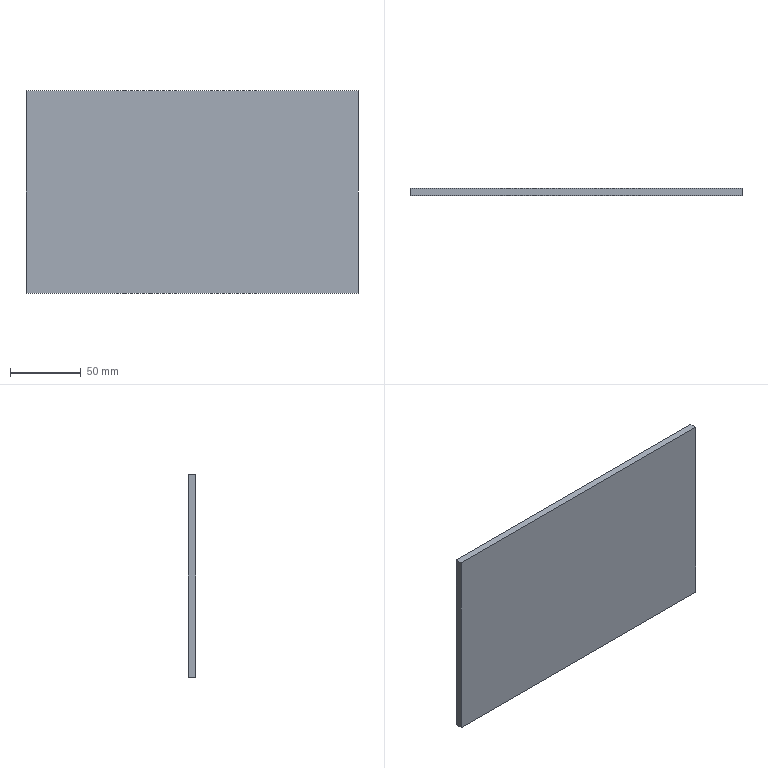Part | SolidWorks | features BaseBody 1 | 1 solid | 6 faces | box 235 x 5 x 143 mm | volume 168025 mm3 | plane 6
STEP:
#1=CARTESIAN_POINT('',(118.5,-5.,71.5));
#2=VERTEX_POINT('',#1);
#3=CARTESIAN_POINT('',(118.5,-5.,-71.5));
#4=VERTEX_POINT('',#3);
#5=CARTESIAN_POINT('',(118.5,-5.,0.));
#6=DIRECTION('',(0.,0.,-1.));
#7=VECTOR('',#6,1000.);
#8=LINE('',#5,#7);
#9=EDGE_CURVE('',#2,#4,#8,.T.);
#10=ORIENTED_EDGE('',*,*,#9,.F.);
#11=CARTESIAN_POINT('',(-116.5,-5.,71.5));
#12=VERTEX_POINT('',#11);
#13=CARTESIAN_POINT('',(0.,-5.,71.5));
#14=DIRECTION('',(1.,0.,0.));
#15=VECTOR('',#14,1000.);
#16=LINE('',#13,#15);
#17=EDGE_CURVE('',#12,#2,#16,.T.);
#18=ORIENTED_EDGE('',*,*,#17,.F.);
#19=CARTESIAN_POINT('',(-116.5,-5.,-71.5));
#20=VERTEX_POINT('',#19);
#21=CARTESIAN_POINT('',(-116.5,-5.,0.));
#22=DIRECTION('',(0.,0.,1.));
#23=VECTOR('',#22,1000.);
#24=LINE('',#21,#23);
#25=EDGE_CURVE('',#20,#12,#24,.T.);
#26=ORIENTED_EDGE('',*,*,#25,.F.);
#27=CARTESIAN_POINT('',(0.,-5.,-71.5));
#28=DIRECTION('',(-1.,0.,0.));
#29=VECTOR('',#28,1000.);
#30=LINE('',#27,#29);
#31=EDGE_CURVE('',#4,#20,#30,.T.);
#32=ORIENTED_EDGE('',*,*,#31,.F.);
#33=EDGE_LOOP('',(#10,#18,#26,#32));
#34=FACE_OUTER_BOUND('',#33,.T.);
#35=CARTESIAN_POINT('',(0.,-5.,0.));
#36=DIRECTION('',(0.,1.,0.));
#37=DIRECTION('',(0.,0.,1.));
#38=AXIS2_PLACEMENT_3D('',#35,#36,#37);
#39=PLANE('',#38);
#40=ADVANCED_FACE('',(#34),#39,.F.);
#41=CARTESIAN_POINT('',(-116.5,0.,-71.5));
#42=VERTEX_POINT('',#41);
#43=CARTESIAN_POINT('',(-116.5,0.,-71.5));
#44=DIRECTION('',(0.,1.,0.));
#45=VECTOR('',#44,1000.);
#46=LINE('',#43,#45);
#47=EDGE_CURVE('',#20,#42,#46,.T.);
#48=ORIENTED_EDGE('',*,*,#47,.T.);
#49=CARTESIAN_POINT('',(118.5,0.,-71.5));
#50=VERTEX_POINT('',#49);
#51=CARTESIAN_POINT('',(118.5,0.,-71.5));
#52=DIRECTION('',(1.,0.,0.));
#53=VECTOR('',#52,1000.);
#54=LINE('',#51,#53);
#55=EDGE_CURVE('',#42,#50,#54,.T.);
#56=ORIENTED_EDGE('',*,*,#55,.T.);
#57=CARTESIAN_POINT('',(118.5,0.,-71.5));
#58=DIRECTION('',(0.,-1.,0.));
#59=VECTOR('',#58,1000.);
#60=LINE('',#57,#59);
#61=EDGE_CURVE('',#50,#4,#60,.T.);
#62=ORIENTED_EDGE('',*,*,#61,.T.);
#63=ORIENTED_EDGE('',*,*,#31,.T.);
#64=EDGE_LOOP('',(#48,#56,#62,#63));
#65=FACE_OUTER_BOUND('',#64,.T.);
#66=CARTESIAN_POINT('',(118.5,0.,-71.5));
#67=DIRECTION('',(0.,0.,-1.));
#68=DIRECTION('',(-1.,0.,0.));
#69=AXIS2_PLACEMENT_3D('',#66,#67,#68);
#70=PLANE('',#69);
#71=ADVANCED_FACE('',(#65),#70,.T.);
#72=ORIENTED_EDGE('',*,*,#61,.F.);
#73=CARTESIAN_POINT('',(118.5,0.,71.5));
#74=VERTEX_POINT('',#73);
#75=CARTESIAN_POINT('',(118.5,0.,71.5));
#76=DIRECTION('',(0.,0.,1.));
#77=VECTOR('',#76,1000.);
#78=LINE('',#75,#77);
#79=EDGE_CURVE('',#50,#74,#78,.T.);
#80=ORIENTED_EDGE('',*,*,#79,.T.);
#81=CARTESIAN_POINT('',(118.5,0.,71.5));
#82=DIRECTION('',(0.,-1.,0.));
#83=VECTOR('',#82,1000.);
#84=LINE('',#81,#83);
#85=EDGE_CURVE('',#74,#2,#84,.T.);
#86=ORIENTED_EDGE('',*,*,#85,.T.);
#87=ORIENTED_EDGE('',*,*,#9,.T.);
#88=EDGE_LOOP('',(#72,#80,#86,#87));
#89=FACE_OUTER_BOUND('',#88,.T.);
#90=CARTESIAN_POINT('',(118.5,0.,71.5));
#91=DIRECTION('',(1.,0.,0.));
#92=DIRECTION('',(0.,0.,-1.));
#93=AXIS2_PLACEMENT_3D('',#90,#91,#92);
#94=PLANE('',#93);
#95=ADVANCED_FACE('',(#89),#94,.T.);
#96=ORIENTED_EDGE('',*,*,#85,.F.);
#97=CARTESIAN_POINT('',(-116.5,0.,71.5));
#98=VERTEX_POINT('',#97);
#99=CARTESIAN_POINT('',(-116.5,0.,71.5));
#100=DIRECTION('',(-1.,0.,0.));
#101=VECTOR('',#100,1000.);
#102=LINE('',#99,#101);
#103=EDGE_CURVE('',#74,#98,#102,.T.);
#104=ORIENTED_EDGE('',*,*,#103,.T.);
#105=CARTESIAN_POINT('',(-116.5,0.,71.5));
#106=DIRECTION('',(0.,-1.,0.));
#107=VECTOR('',#106,1000.);
#108=LINE('',#105,#107);
#109=EDGE_CURVE('',#98,#12,#108,.T.);
#110=ORIENTED_EDGE('',*,*,#109,.T.);
#111=ORIENTED_EDGE('',*,*,#17,.T.);
#112=EDGE_LOOP('',(#96,#104,#110,#111));
#113=FACE_OUTER_BOUND('',#112,.T.);
#114=CARTESIAN_POINT('',(-116.5,0.,71.5));
#115=DIRECTION('',(0.,0.,1.));
#116=DIRECTION('',(1.,0.,0.));
#117=AXIS2_PLACEMENT_3D('',#114,#115,#116);
#118=PLANE('',#117);
#119=ADVANCED_FACE('',(#113),#118,.T.);
#120=ORIENTED_EDGE('',*,*,#109,.F.);
#121=CARTESIAN_POINT('',(-116.5,0.,-71.5));
#122=DIRECTION('',(0.,0.,-1.));
#123=VECTOR('',#122,1000.);
#124=LINE('',#121,#123);
#125=EDGE_CURVE('',#98,#42,#124,.T.);
#126=ORIENTED_EDGE('',*,*,#125,.T.);
#127=ORIENTED_EDGE('',*,*,#47,.F.);
#128=ORIENTED_EDGE('',*,*,#25,.T.);
#129=EDGE_LOOP('',(#120,#126,#127,#128));
#130=FACE_OUTER_BOUND('',#129,.T.);
#131=CARTESIAN_POINT('',(-116.5,0.,-71.5));
#132=DIRECTION('',(-1.,0.,0.));
#133=DIRECTION('',(0.,0.,1.));
#134=AXIS2_PLACEMENT_3D('',#131,#132,#133);
#135=PLANE('',#134);
#136=ADVANCED_FACE('',(#130),#135,.T.);
#137=ORIENTED_EDGE('',*,*,#125,.F.);
#138=ORIENTED_EDGE('',*,*,#103,.F.);
#139=ORIENTED_EDGE('',*,*,#79,.F.);
#140=ORIENTED_EDGE('',*,*,#55,.F.);
#141=EDGE_LOOP('',(#137,#138,#139,#140));
#142=FACE_OUTER_BOUND('',#141,.T.);
#143=CARTESIAN_POINT('',(0.,0.,0.));
#144=DIRECTION('',(0.,1.,0.));
#145=DIRECTION('',(0.,0.,1.));
#146=AXIS2_PLACEMENT_3D('',#143,#144,#145);
#147=PLANE('',#146);
#148=ADVANCED_FACE('',(#142),#147,.T.);
#149=CLOSED_SHELL('',(#40,#71,#95,#119,#136,#148));
#150=MANIFOLD_SOLID_BREP('',#149);
#151=CARTESIAN_POINT('',(0.,0.,0.));
#152=DIRECTION('',(0.,0.,1.));
#153=DIRECTION('',(1.,0.,0.));
#154=AXIS2_PLACEMENT_3D('',#151,#152,#153);
#155=(LENGTH_UNIT()NAMED_UNIT(*)SI_UNIT(.MILLI.,.METRE.));
#156=UNCERTAINTY_MEASURE_WITH_UNIT(LENGTH_MEASURE(0.00001),#155,'','');
#157=(NAMED_UNIT(*)PLANE_ANGLE_UNIT()SI_UNIT($,.RADIAN.));
#158=(NAMED_UNIT(*)SI_UNIT($,.STERADIAN.)SOLID_ANGLE_UNIT());
#159=(GEOMETRIC_REPRESENTATION_CONTEXT(3)GLOBAL_UNCERTAINTY_ASSIGNED_CONTEXT((#156))GLOBAL_UNIT_ASSIGNED_CONTEXT((#155,#157,#158))REPRESENTATION_CONTEXT('',''));
#160=ADVANCED_BREP_SHAPE_REPRESENTATION('',(#150,#154),#159);